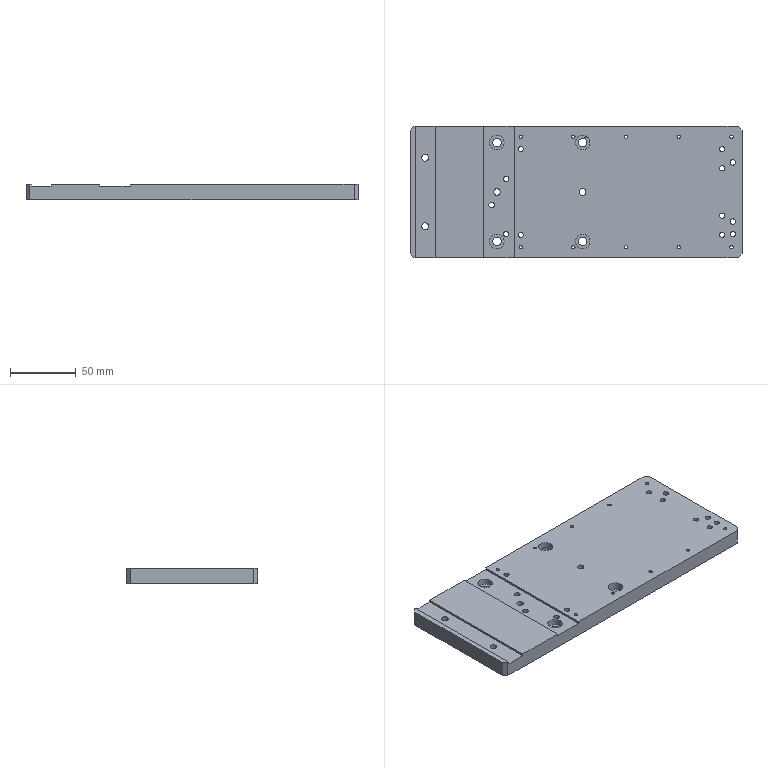Part | 1 solid | 70 faces | box 252 x 100 x 12 mm | volume 289943 mm3 | cylinder 41 | plane 22 | cone 7 | commonest cylinder face diameters 2.5 x16 4 x8 4.2 x4 6.6 x4 11 x4 5 x2